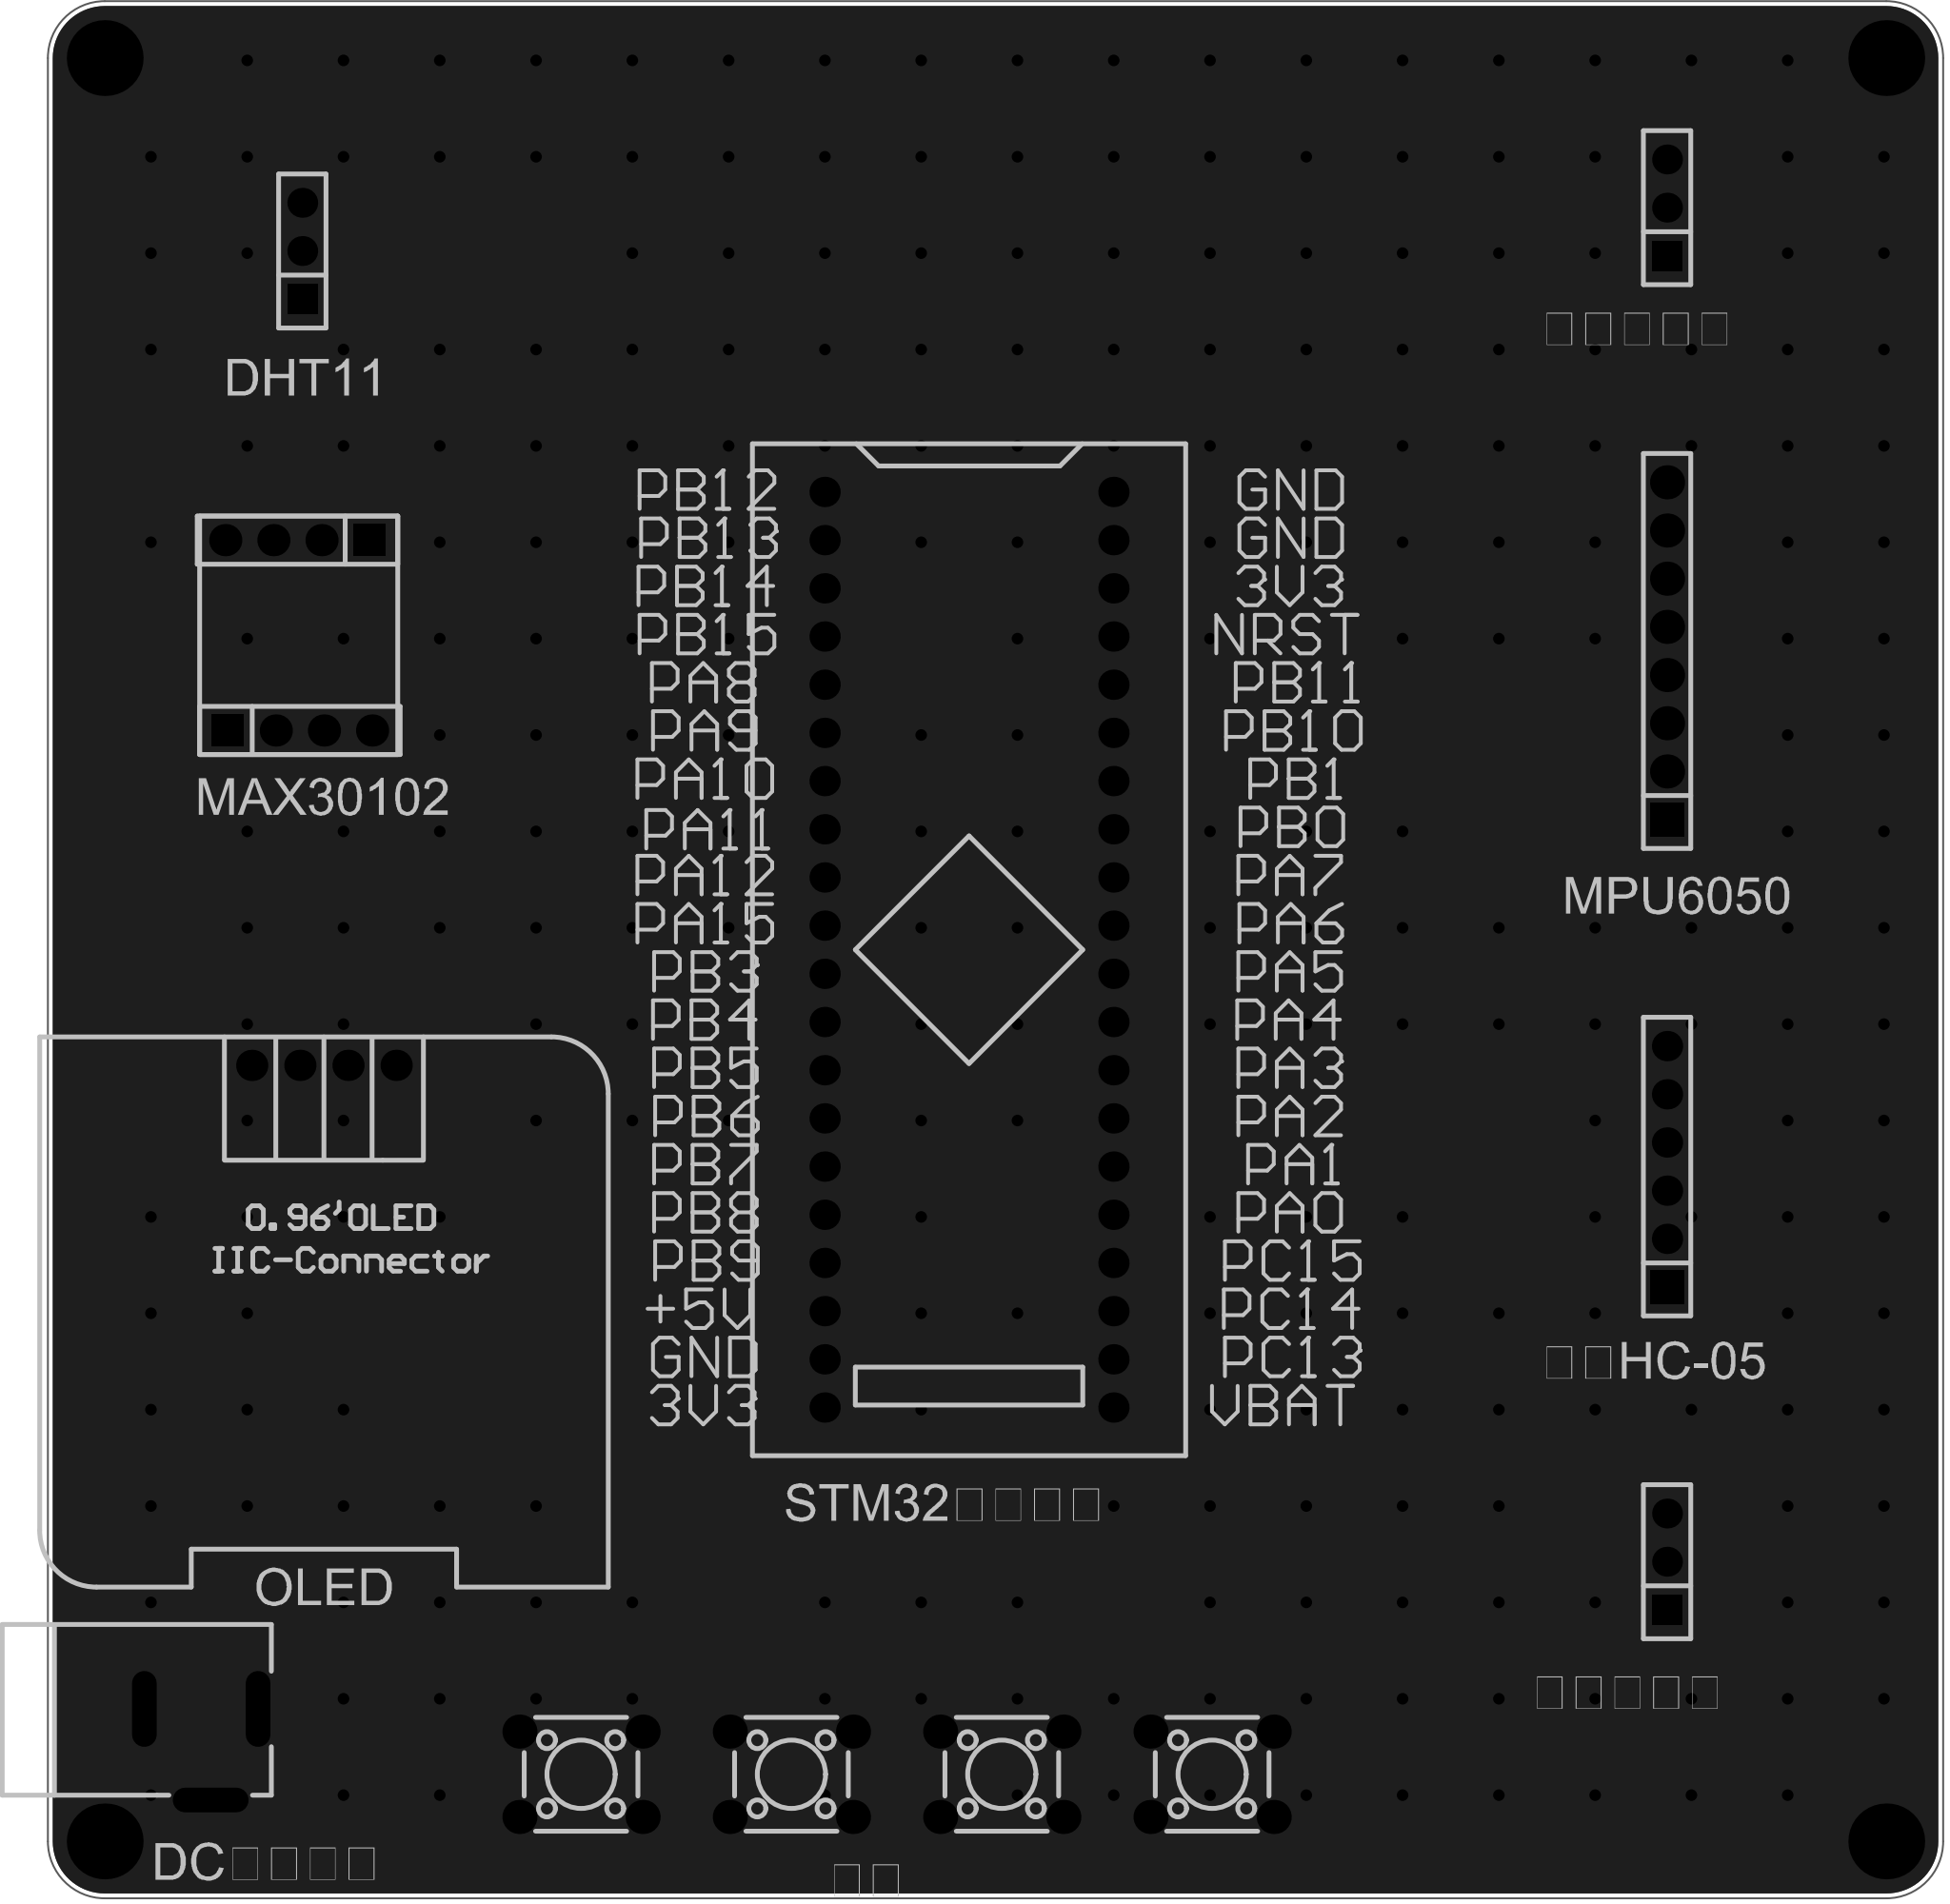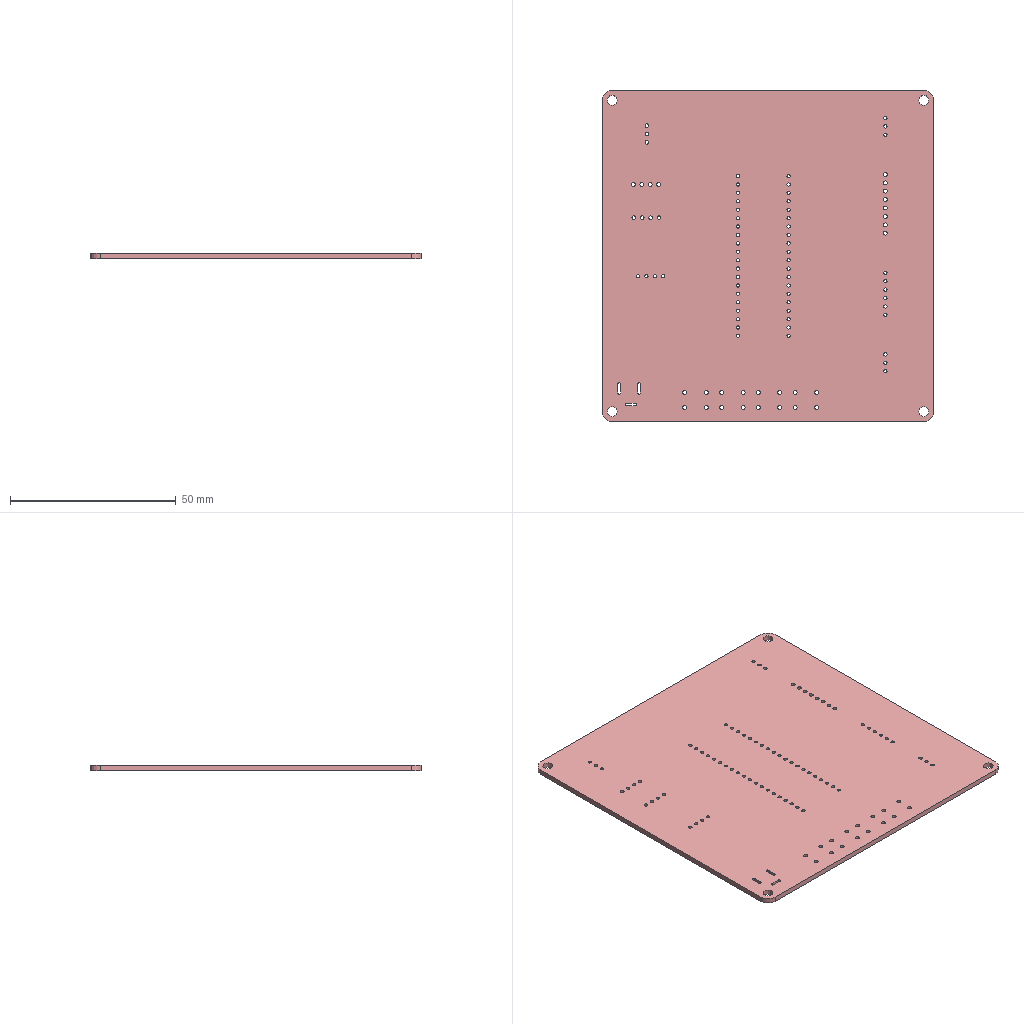Circuit board layout | Altium Designer | box 100 x 100 x 1.6 mm
Layer stack:
# Altium Designer layer stack of  (unit mm; dielectric type: 0 none, 1 core, 2 prepreg, 3 surface material)
index,name,kind,layer,copper_thickness_mm,dielectric_type,dielectric_thickness_mm,dielectric_material,dielectric_constant
0,Top Paste Mask Layer,other,,,,,,
1,Top Silkscreen Layer,other,,,,,,
2,Top Solder Mask Layer,dielectric,,,3,0.01,,3.3
3,Top Layer,copper,Top Layer,0.035,,,,
4,Dielectric1,dielectric,,,3,1.51,FR4,4.5
5,Bottom Layer,copper,Bottom Layer,0.035,,,,
6,Bottom Solder Mask Layer,dielectric,,,3,0.01,,3.3
7,Bottom Silkscreen Layer,other,,,,,,
8,Bottom Paste Mask Layer,other,,,,,,
# drill layer pairs: low layer,high layer
drill_pair,Top Layer,Bottom Layer
Part placement:
Designator,Comment,Layer,Footprint,Center-X(mm),Center-Y(mm),Rotation
U1,STM32F103C8T6-Card,TopLayer,CONN-TH_L53.3-W22.9_STM32F103C8T6-CARD,129.159,128.905,270
H13,,TopLayer,HDR-TH_4P-P2.54-V-F,93.853,140.462,0
H12,,TopLayer,HDR-TH_4P-P2.54-V-F,93.726,150.495,180
H1,,TopLayer,HDR-TH_3P-P2.54-V-F,165.989,96.647,90
H2,,TopLayer,HDR-TH_8P-P2.54-V-F-1,165.989,144.653,90
DC1,,TopLayer,DC-2.0,88.646,86.487,180
H3,,TopLayer,HDR-TH_3P-P2.54-V-F,93.98,165.735,90
H4,,TopLayer,HDR-TH_6P-P2.54-V-F,165.989,117.475,90
H5,,TopLayer,HDR-TH_3P-P2.54-V-F,165.989,168.021,90
OLED1,,TopLayer,0.96OLED_4P,95.123,122.809,0
SW1,,TopLayer,SW-TH_4P-L6.0-W6.0-P4.50-LS6.5,141.986,85.443,0
SW2,,TopLayer,SW-TH_4P-L6.0-W6.0-P4.50-LS6.5,130.887,85.443,0
SW3,,TopLayer,SW-TH_4P-L6.0-W6.0-P4.50-LS6.5,119.787,85.443,0
SW4,,TopLayer,SW-TH_4P-L6.0-W6.0-P4.50-LS6.5,108.688,85.443,0
Pad and via stacks:
# Altium Designer via and pad stacks of  (unit mm). Each distinct definition once, with the count of objects using it.
# via: kind,start_layer,end_layer,hole_mm,diameter_mm,mode(0 simple;1 top-mid-bottom;2 full stack),diameter_per_layer,count,example_net
# pad: kind,layer,hole_mm,hole_type(0 round;1 square;2 slot),plating,top_size,top_shape(1 round;2 rect;3 octagon;9 rounded rect),mid_size,bottom_size,mode,footprint,size_per_layer,count,example
pad,Multi-Layer,3,0,plated,4x4,1,4x4,4x4,0,,,4,1
pad,Multi-Layer,1,0,plated,1.6x1.6,1,1.6x1.6,1.6x1.6,0,CONN-TH_L53.3-W22.9_STM32F103C8T6-CARD,,40,U1.1
pad,Multi-Layer,1.1,0,plated,1.7x1.7,2,1.7x1.7,1.7x1.7,0,HDR-TH_4P-P2.54-V-F,,2,H13.1
pad,Multi-Layer,1.1,0,plated,1.7x1.7,1,1.7x1.7,1.7x1.7,0,HDR-TH_4P-P2.54-V-F,,6,H13.2
pad,Multi-Layer,1.02,0,plated,1.575x1.575,1,1.575x1.575,1.575x1.575,0,HDR-TH_3P-P2.54-V-F,,6,H1.3
pad,Multi-Layer,1.02,0,plated,1.575x1.575,2,1.575x1.575,1.575x1.575,0,HDR-TH_3P-P2.54-V-F,,3,H1.1
pad,Multi-Layer,1.2,0,plated,1.8x1.8,2,1.8x1.8,1.8x1.8,0,HDR-TH_8P-P2.54-V-F-1,,1,H2.1
pad,Multi-Layer,1.2,0,plated,1.8x1.8,1,1.8x1.8,1.8x1.8,0,HDR-TH_8P-P2.54-V-F-1,,7,H2.2
pad,Multi-Layer,0.8001,2,plated,4x1.3,1,4x1.3,4x1.3,0,DC-2.0,,3,DC1.2
pad,Multi-Layer,1.02,0,plated,1.6x1.6,1,1.6x1.6,1.6x1.6,0,HDR-TH_6P-P2.54-V-F,,5,H4.6
pad,Multi-Layer,1.02,0,plated,1.8x1.8,2,1.8x1.8,1.8x1.8,0,HDR-TH_6P-P2.54-V-F,,1,H4.1
pad,Multi-Layer,1,0,plated,1.65x1.65,1,1.65x1.65,1.65x1.65,0,0.96OLED_4P,,4,OLED1.4
pad,Multi-Layer,1.2,0,plated,1.8x1.8,1,1.8x1.8,1.8x1.8,0,SW-TH_4P-L6.0-W6.0-P4.50-LS6.5,,16,SW1.1
via,Top Layer,Bottom Layer,0.3048,0.61,0,,265,GND
Copper pours:
name,layer,net,type(0 solid;1 hatched;2 none)
Bottom Layer-GND,Bottom Layer,GND,0
Top Layer-GND,Top Layer,GND,0
Design rules, without the lines most boards share:
# Altium Designer design rules of  (exported by Altium Designer, unit mm)
# columns: name | kind | enabled | priority | scope1 | scope2 | descriptor | typed fields (field=value)
copperThickness1oz_2 | 2 | enabled | 2 | All | All | Width Constraint (Min=5mil) (Max=100mil) (Preferred=30mil) (All) |
viaSize | 11 | enabled | 1 | All | All | Routing Via (MinHoleWidth=11.811mil) (MaxHoleWidth=248.032mil) (PreferredHoleWidth=12.008mil) (MinWidth=19.685mil) (MaxWidth=393.701mil) (PreferedWidth=24.016mil) (All) | via_min_hole=0.3 via_max_hole=6.3 via_preferred_diameter=0.61 via_preferred_hole=0.305
solderMaskExpansion | 13 | enabled | 2 | All | All | Solder Mask Expansion (Expansion =2.008mil) (All) | expansion=0.051